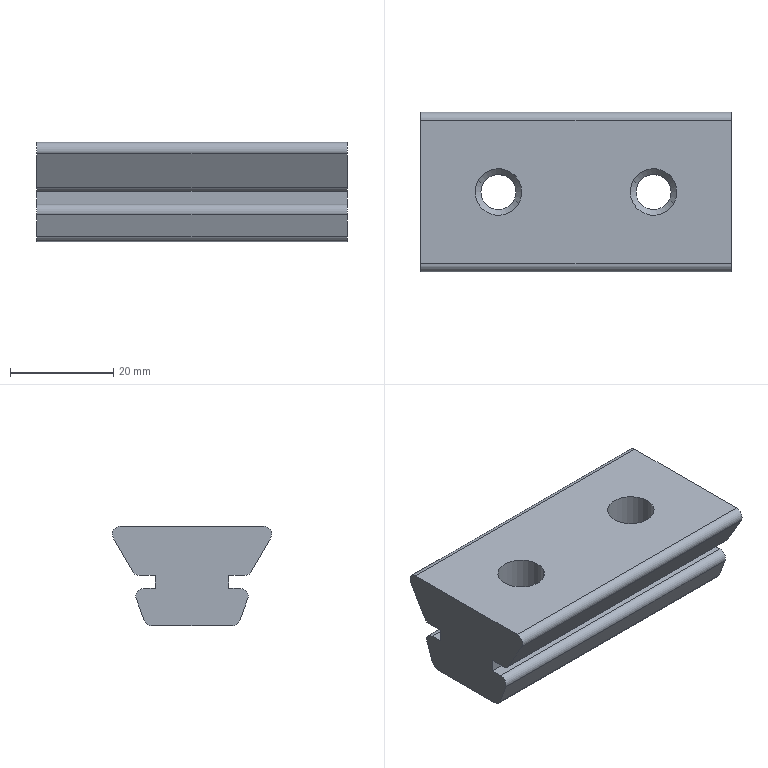Part | STEP file | 31E-01014QY25 | 1 solid | 34 faces | box 60 x 30.804 x 19.2 mm | volume 24408 mm3 | cylinder 16 | plane 14 | cone 4 | commonest cylinder face diameters 3 x8 6.8 x4 9 x4
STEP:
#1=CARTESIAN_POINT('',(0.,-7.1,-9.5));
#2=VERTEX_POINT('',#1);
#3=CARTESIAN_POINT('',(60.,-7.1,-9.5));
#4=VERTEX_POINT('',#3);
#5=CARTESIAN_POINT('',(30.,-7.1,-9.5));
#6=DIRECTION('',(1.,0.,0.));
#7=VECTOR('',#6,1.);
#8=LINE('',#5,#7);
#9=EDGE_CURVE('',#2,#4,#8,.T.);
#10=ORIENTED_EDGE('',*,*,#9,.F.);
#11=CARTESIAN_POINT('',(0.,-7.1,-12.));
#12=VERTEX_POINT('',#11);
#13=CARTESIAN_POINT('',(0.,-7.1,-10.75));
#14=DIRECTION('',(0.,0.,-1.));
#15=VECTOR('',#14,1.);
#16=LINE('',#13,#15);
#17=EDGE_CURVE('',#2,#12,#16,.T.);
#18=ORIENTED_EDGE('',*,*,#17,.T.);
#19=CARTESIAN_POINT('',(60.,-7.1,-12.));
#20=VERTEX_POINT('',#19);
#21=CARTESIAN_POINT('',(30.,-7.1,-12.));
#22=DIRECTION('',(1.,0.,0.));
#23=VECTOR('',#22,1.);
#24=LINE('',#21,#23);
#25=EDGE_CURVE('',#12,#20,#24,.T.);
#26=ORIENTED_EDGE('',*,*,#25,.T.);
#27=CARTESIAN_POINT('',(60.,-7.1,-10.75));
#28=DIRECTION('',(0.,0.,-1.));
#29=VECTOR('',#28,1.);
#30=LINE('',#27,#29);
#31=EDGE_CURVE('',#4,#20,#30,.T.);
#32=ORIENTED_EDGE('',*,*,#31,.F.);
#33=EDGE_LOOP('',(#10,#18,#26,#32));
#34=FACE_OUTER_BOUND('',#33,.T.);
#35=CARTESIAN_POINT('',(0.,-7.1,-9.5));
#36=DIRECTION('',(0.,-1.,0.));
#37=DIRECTION('',(0.,0.,-1.));
#38=AXIS2_PLACEMENT_3D('',#35,#36,#37);
#39=PLANE('',#38);
#40=ADVANCED_FACE('',(#34),#39,.T.);
#41=CARTESIAN_POINT('',(0.,7.1,-12.));
#42=VERTEX_POINT('',#41);
#43=CARTESIAN_POINT('',(60.,7.1,-12.));
#44=VERTEX_POINT('',#43);
#45=CARTESIAN_POINT('',(30.,7.1,-12.));
#46=DIRECTION('',(1.,0.,0.));
#47=VECTOR('',#46,1.);
#48=LINE('',#45,#47);
#49=EDGE_CURVE('',#42,#44,#48,.T.);
#50=ORIENTED_EDGE('',*,*,#49,.F.);
#51=CARTESIAN_POINT('',(0.,7.1,-9.5));
#52=VERTEX_POINT('',#51);
#53=CARTESIAN_POINT('',(0.,7.1,-10.75));
#54=DIRECTION('',(0.,0.,-1.));
#55=VECTOR('',#54,1.);
#56=LINE('',#53,#55);
#57=EDGE_CURVE('',#42,#52,#56,.F.);
#58=ORIENTED_EDGE('',*,*,#57,.T.);
#59=CARTESIAN_POINT('',(60.,7.1,-9.5));
#60=VERTEX_POINT('',#59);
#61=CARTESIAN_POINT('',(30.,7.1,-9.5));
#62=DIRECTION('',(1.,0.,0.));
#63=VECTOR('',#62,1.);
#64=LINE('',#61,#63);
#65=EDGE_CURVE('',#52,#60,#64,.T.);
#66=ORIENTED_EDGE('',*,*,#65,.T.);
#67=CARTESIAN_POINT('',(60.,7.1,-10.75));
#68=DIRECTION('',(0.,0.,-1.));
#69=VECTOR('',#68,1.);
#70=LINE('',#67,#69);
#71=EDGE_CURVE('',#44,#60,#70,.F.);
#72=ORIENTED_EDGE('',*,*,#71,.F.);
#73=EDGE_LOOP('',(#50,#58,#66,#72));
#74=FACE_OUTER_BOUND('',#73,.T.);
#75=CARTESIAN_POINT('',(0.,7.1,-9.5));
#76=DIRECTION('',(0.,-1.,0.));
#77=DIRECTION('',(0.,0.,-1.));
#78=AXIS2_PLACEMENT_3D('',#75,#76,#77);
#79=PLANE('',#78);
#80=ADVANCED_FACE('',(#74),#79,.F.);
#81=CARTESIAN_POINT('',(60.,13.902,0.));
#82=VERTEX_POINT('',#81);
#83=CARTESIAN_POINT('',(60.,15.201,-2.25));
#84=VERTEX_POINT('',#83);
#85=CARTESIAN_POINT('',(60.,13.902,-1.5));
#86=DIRECTION('',(1.,0.,0.));
#87=AXIS2_PLACEMENT_3D('',#85,#86,$);
#88=CIRCLE('',#87,1.5);
#89=EDGE_CURVE('',#82,#84,#88,.F.);
#90=ORIENTED_EDGE('',*,*,#89,.T.);
#91=CARTESIAN_POINT('',(0.,15.201,-2.25));
#92=VERTEX_POINT('',#91);
#93=CARTESIAN_POINT('',(30.,15.201,-2.25));
#94=DIRECTION('',(1.,0.,0.));
#95=VECTOR('',#94,1.);
#96=LINE('',#93,#95);
#97=EDGE_CURVE('',#92,#84,#96,.T.);
#98=ORIENTED_EDGE('',*,*,#97,.F.);
#99=CARTESIAN_POINT('',(0.,13.902,0.));
#100=VERTEX_POINT('',#99);
#101=CARTESIAN_POINT('',(0.,13.902,-1.5));
#102=DIRECTION('',(1.,0.,0.));
#103=AXIS2_PLACEMENT_3D('',#101,#102,$);
#104=CIRCLE('',#103,1.5);
#105=EDGE_CURVE('',#92,#100,#104,.T.);
#106=ORIENTED_EDGE('',*,*,#105,.T.);
#107=CARTESIAN_POINT('',(30.,13.902,0.));
#108=DIRECTION('',(1.,0.,0.));
#109=VECTOR('',#108,1.);
#110=LINE('',#107,#109);
#111=EDGE_CURVE('',#100,#82,#110,.T.);
#112=ORIENTED_EDGE('',*,*,#111,.T.);
#113=EDGE_LOOP('',(#90,#98,#106,#112));
#114=FACE_OUTER_BOUND('',#113,.T.);
#115=CARTESIAN_POINT('',(30.,13.902,-1.5));
#116=DIRECTION('',(1.,0.,0.));
#117=DIRECTION('',(0.,0.866,-0.5));
#118=AXIS2_PLACEMENT_3D('',#115,#116,#117);
#119=CYLINDRICAL_SURFACE('',#118,1.5);
#120=ADVANCED_FACE('',(#114),#119,.T.);
#121=CARTESIAN_POINT('',(60.,-15.201,-2.25));
#122=VERTEX_POINT('',#121);
#123=CARTESIAN_POINT('',(60.,-13.902,0.));
#124=VERTEX_POINT('',#123);
#125=CARTESIAN_POINT('',(60.,-13.902,-1.5));
#126=DIRECTION('',(1.,0.,0.));
#127=AXIS2_PLACEMENT_3D('',#125,#126,$);
#128=CIRCLE('',#127,1.5);
#129=EDGE_CURVE('',#122,#124,#128,.F.);
#130=ORIENTED_EDGE('',*,*,#129,.T.);
#131=CARTESIAN_POINT('',(0.,-13.902,0.));
#132=VERTEX_POINT('',#131);
#133=CARTESIAN_POINT('',(30.,-13.902,0.));
#134=DIRECTION('',(1.,0.,0.));
#135=VECTOR('',#134,1.);
#136=LINE('',#133,#135);
#137=EDGE_CURVE('',#132,#124,#136,.T.);
#138=ORIENTED_EDGE('',*,*,#137,.F.);
#139=CARTESIAN_POINT('',(0.,-15.201,-2.25));
#140=VERTEX_POINT('',#139);
#141=CARTESIAN_POINT('',(0.,-13.902,-1.5));
#142=DIRECTION('',(1.,0.,0.));
#143=AXIS2_PLACEMENT_3D('',#141,#142,$);
#144=CIRCLE('',#143,1.5);
#145=EDGE_CURVE('',#132,#140,#144,.T.);
#146=ORIENTED_EDGE('',*,*,#145,.T.);
#147=CARTESIAN_POINT('',(30.,-15.201,-2.25));
#148=DIRECTION('',(1.,0.,0.));
#149=VECTOR('',#148,1.);
#150=LINE('',#147,#149);
#151=EDGE_CURVE('',#140,#122,#150,.T.);
#152=ORIENTED_EDGE('',*,*,#151,.T.);
#153=EDGE_LOOP('',(#130,#138,#146,#152));
#154=FACE_OUTER_BOUND('',#153,.T.);
#155=CARTESIAN_POINT('',(30.,-13.902,-1.5));
#156=DIRECTION('',(1.,0.,0.));
#157=DIRECTION('',(0.,0.,1.));
#158=AXIS2_PLACEMENT_3D('',#155,#156,#157);
#159=CYLINDRICAL_SURFACE('',#158,1.5);
#160=ADVANCED_FACE('',(#154),#159,.T.);
#161=CARTESIAN_POINT('',(60.,10.149,-9.5));
#162=VERTEX_POINT('',#161);
#163=CARTESIAN_POINT('',(60.,8.625,-9.5));
#164=DIRECTION('',(0.,-1.,0.));
#165=VECTOR('',#164,1.);
#166=LINE('',#163,#165);
#167=EDGE_CURVE('',#60,#162,#166,.F.);
#168=ORIENTED_EDGE('',*,*,#167,.F.);
#169=ORIENTED_EDGE('',*,*,#65,.F.);
#170=CARTESIAN_POINT('',(0.,10.149,-9.5));
#171=VERTEX_POINT('',#170);
#172=CARTESIAN_POINT('',(0.,8.625,-9.5));
#173=DIRECTION('',(0.,-1.,0.));
#174=VECTOR('',#173,1.);
#175=LINE('',#172,#174);
#176=EDGE_CURVE('',#52,#171,#175,.F.);
#177=ORIENTED_EDGE('',*,*,#176,.T.);
#178=CARTESIAN_POINT('',(30.,10.149,-9.5));
#179=DIRECTION('',(1.,0.,0.));
#180=VECTOR('',#179,1.);
#181=LINE('',#178,#180);
#182=EDGE_CURVE('',#171,#162,#181,.T.);
#183=ORIENTED_EDGE('',*,*,#182,.T.);
#184=EDGE_LOOP('',(#168,#169,#177,#183));
#185=FACE_OUTER_BOUND('',#184,.T.);
#186=CARTESIAN_POINT('',(0.,-11.015,-9.5));
#187=DIRECTION('',(0.,0.,-1.));
#188=DIRECTION('',(0.,1.,0.));
#189=AXIS2_PLACEMENT_3D('',#186,#187,#188);
#190=PLANE('',#189);
#191=ADVANCED_FACE('',(#185),#190,.T.);
#192=CARTESIAN_POINT('',(0.,11.448,-8.75));
#193=VERTEX_POINT('',#192);
#194=CARTESIAN_POINT('',(60.,11.448,-8.75));
#195=VERTEX_POINT('',#194);
#196=CARTESIAN_POINT('',(30.,11.448,-8.75));
#197=DIRECTION('',(1.,0.,0.));
#198=VECTOR('',#197,1.);
#199=LINE('',#196,#198);
#200=EDGE_CURVE('',#193,#195,#199,.T.);
#201=ORIENTED_EDGE('',*,*,#200,.F.);
#202=CARTESIAN_POINT('',(0.,13.325,-5.5));
#203=DIRECTION('',(0.,-0.5,-0.866));
#204=VECTOR('',#203,1.);
#205=LINE('',#202,#204);
#206=EDGE_CURVE('',#193,#92,#205,.F.);
#207=ORIENTED_EDGE('',*,*,#206,.T.);
#208=ORIENTED_EDGE('',*,*,#97,.T.);
#209=CARTESIAN_POINT('',(60.,13.325,-5.5));
#210=DIRECTION('',(0.,-0.5,-0.866));
#211=VECTOR('',#210,1.);
#212=LINE('',#209,#211);
#213=EDGE_CURVE('',#195,#84,#212,.F.);
#214=ORIENTED_EDGE('',*,*,#213,.F.);
#215=EDGE_LOOP('',(#201,#207,#208,#214));
#216=FACE_OUTER_BOUND('',#215,.T.);
#217=CARTESIAN_POINT('',(0.,16.5,0.));
#218=DIRECTION('',(0.,-0.866,0.5));
#219=DIRECTION('',(0.,-0.5,-0.866));
#220=AXIS2_PLACEMENT_3D('',#217,#218,#219);
#221=PLANE('',#220);
#222=ADVANCED_FACE('',(#216),#221,.F.);
#223=CARTESIAN_POINT('',(60.,10.149,-8.));
#224=DIRECTION('',(1.,0.,0.));
#225=AXIS2_PLACEMENT_3D('',#223,#224,$);
#226=CIRCLE('',#225,1.5);
#227=EDGE_CURVE('',#195,#162,#226,.F.);
#228=ORIENTED_EDGE('',*,*,#227,.T.);
#229=ORIENTED_EDGE('',*,*,#182,.F.);
#230=CARTESIAN_POINT('',(0.,10.149,-8.));
#231=DIRECTION('',(1.,0.,0.));
#232=AXIS2_PLACEMENT_3D('',#230,#231,$);
#233=CIRCLE('',#232,1.5);
#234=EDGE_CURVE('',#171,#193,#233,.T.);
#235=ORIENTED_EDGE('',*,*,#234,.T.);
#236=ORIENTED_EDGE('',*,*,#200,.T.);
#237=EDGE_LOOP('',(#228,#229,#235,#236));
#238=FACE_OUTER_BOUND('',#237,.T.);
#239=CARTESIAN_POINT('',(30.,10.149,-8.));
#240=DIRECTION('',(1.,0.,0.));
#241=DIRECTION('',(0.,0.,-1.));
#242=AXIS2_PLACEMENT_3D('',#239,#240,#241);
#243=CYLINDRICAL_SURFACE('',#242,1.5);
#244=ADVANCED_FACE('',(#238),#243,.T.);
#245=CARTESIAN_POINT('',(0.,9.358,-12.));
#246=VERTEX_POINT('',#245);
#247=CARTESIAN_POINT('',(0.,8.229,-12.));
#248=DIRECTION('',(0.,1.,0.));
#249=VECTOR('',#248,1.);
#250=LINE('',#247,#249);
#251=EDGE_CURVE('',#246,#42,#250,.F.);
#252=ORIENTED_EDGE('',*,*,#251,.T.);
#253=ORIENTED_EDGE('',*,*,#49,.T.);
#254=CARTESIAN_POINT('',(60.,9.358,-12.));
#255=VERTEX_POINT('',#254);
#256=CARTESIAN_POINT('',(60.,8.229,-12.));
#257=DIRECTION('',(0.,1.,0.));
#258=VECTOR('',#257,1.);
#259=LINE('',#256,#258);
#260=EDGE_CURVE('',#255,#44,#259,.F.);
#261=ORIENTED_EDGE('',*,*,#260,.F.);
#262=CARTESIAN_POINT('',(30.,9.358,-12.));
#263=DIRECTION('',(1.,0.,0.));
#264=VECTOR('',#263,1.);
#265=LINE('',#262,#264);
#266=EDGE_CURVE('',#246,#255,#265,.T.);
#267=ORIENTED_EDGE('',*,*,#266,.F.);
#268=EDGE_LOOP('',(#252,#253,#261,#267));
#269=FACE_OUTER_BOUND('',#268,.T.);
#270=CARTESIAN_POINT('',(0.,-7.1,-12.));
#271=DIRECTION('',(0.,0.,1.));
#272=DIRECTION('',(0.,-1.,0.));
#273=AXIS2_PLACEMENT_3D('',#270,#271,#272);
#274=PLANE('',#273);
#275=ADVANCED_FACE('',(#269),#274,.T.);
#276=CARTESIAN_POINT('',(60.,10.767,-14.013));
#277=VERTEX_POINT('',#276);
#278=CARTESIAN_POINT('',(60.,9.358,-13.5));
#279=DIRECTION('',(1.,0.,0.));
#280=AXIS2_PLACEMENT_3D('',#278,#279,$);
#281=CIRCLE('',#280,1.5);
#282=EDGE_CURVE('',#255,#277,#281,.F.);
#283=ORIENTED_EDGE('',*,*,#282,.T.);
#284=CARTESIAN_POINT('',(0.,10.767,-14.013));
#285=VERTEX_POINT('',#284);
#286=CARTESIAN_POINT('',(30.,10.767,-14.013));
#287=DIRECTION('',(1.,0.,0.));
#288=VECTOR('',#287,1.);
#289=LINE('',#286,#288);
#290=EDGE_CURVE('',#285,#277,#289,.T.);
#291=ORIENTED_EDGE('',*,*,#290,.F.);
#292=CARTESIAN_POINT('',(0.,9.358,-13.5));
#293=DIRECTION('',(1.,0.,0.));
#294=AXIS2_PLACEMENT_3D('',#292,#293,$);
#295=CIRCLE('',#294,1.5);
#296=EDGE_CURVE('',#285,#246,#295,.T.);
#297=ORIENTED_EDGE('',*,*,#296,.T.);
#298=ORIENTED_EDGE('',*,*,#266,.T.);
#299=EDGE_LOOP('',(#283,#291,#297,#298));
#300=FACE_OUTER_BOUND('',#299,.T.);
#301=CARTESIAN_POINT('',(30.,9.358,-13.5));
#302=DIRECTION('',(1.,0.,0.));
#303=DIRECTION('',(0.,0.9397,-0.342));
#304=AXIS2_PLACEMENT_3D('',#301,#302,#303);
#305=CYLINDRICAL_SURFACE('',#304,1.5);
#306=ADVANCED_FACE('',(#300),#305,.T.);
#307=CARTESIAN_POINT('',(0.,9.239,-18.213));
#308=VERTEX_POINT('',#307);
#309=CARTESIAN_POINT('',(60.,9.239,-18.213));
#310=VERTEX_POINT('',#309);
#311=CARTESIAN_POINT('',(30.,9.239,-18.213));
#312=DIRECTION('',(1.,0.,0.));
#313=VECTOR('',#312,1.);
#314=LINE('',#311,#313);
#315=EDGE_CURVE('',#308,#310,#314,.T.);
#316=ORIENTED_EDGE('',*,*,#315,.F.);
#317=CARTESIAN_POINT('',(0.,10.003,-16.113));
#318=DIRECTION('',(0.,-0.342,-0.9397));
#319=VECTOR('',#318,1.);
#320=LINE('',#317,#319);
#321=EDGE_CURVE('',#308,#285,#320,.F.);
#322=ORIENTED_EDGE('',*,*,#321,.T.);
#323=ORIENTED_EDGE('',*,*,#290,.T.);
#324=CARTESIAN_POINT('',(60.,10.003,-16.113));
#325=DIRECTION('',(0.,-0.342,-0.9397));
#326=VECTOR('',#325,1.);
#327=LINE('',#324,#326);
#328=EDGE_CURVE('',#310,#277,#327,.F.);
#329=ORIENTED_EDGE('',*,*,#328,.F.);
#330=EDGE_LOOP('',(#316,#322,#323,#329));
#331=FACE_OUTER_BOUND('',#330,.T.);
#332=CARTESIAN_POINT('',(0.,11.5,-12.));
#333=DIRECTION('',(0.,-0.9397,0.342));
#334=DIRECTION('',(0.,-0.342,-0.9397));
#335=AXIS2_PLACEMENT_3D('',#332,#333,#334);
#336=PLANE('',#335);
#337=ADVANCED_FACE('',(#331),#336,.F.);
#338=CARTESIAN_POINT('',(60.,7.829,-19.2));
#339=VERTEX_POINT('',#338);
#340=CARTESIAN_POINT('',(60.,7.829,-17.7));
#341=DIRECTION('',(1.,0.,0.));
#342=AXIS2_PLACEMENT_3D('',#340,#341,$);
#343=CIRCLE('',#342,1.5);
#344=EDGE_CURVE('',#310,#339,#343,.F.);
#345=ORIENTED_EDGE('',*,*,#344,.T.);
#346=CARTESIAN_POINT('',(0.,7.829,-19.2));
#347=VERTEX_POINT('',#346);
#348=CARTESIAN_POINT('',(30.,7.829,-19.2));
#349=DIRECTION('',(1.,0.,0.));
#350=VECTOR('',#349,1.);
#351=LINE('',#348,#350);
#352=EDGE_CURVE('',#347,#339,#351,.T.);
#353=ORIENTED_EDGE('',*,*,#352,.F.);
#354=CARTESIAN_POINT('',(0.,7.829,-17.7));
#355=DIRECTION('',(1.,0.,0.));
#356=AXIS2_PLACEMENT_3D('',#354,#355,$);
#357=CIRCLE('',#356,1.5);
#358=EDGE_CURVE('',#347,#308,#357,.T.);
#359=ORIENTED_EDGE('',*,*,#358,.T.);
#360=ORIENTED_EDGE('',*,*,#315,.T.);
#361=EDGE_LOOP('',(#345,#353,#359,#360));
#362=FACE_OUTER_BOUND('',#361,.T.);
#363=CARTESIAN_POINT('',(30.,7.829,-17.7));
#364=DIRECTION('',(1.,0.,0.));
#365=DIRECTION('',(0.,0.,-1.));
#366=AXIS2_PLACEMENT_3D('',#363,#364,#365);
#367=CYLINDRICAL_SURFACE('',#366,1.5);
#368=ADVANCED_FACE('',(#362),#367,.T.);
#369=CARTESIAN_POINT('',(60.,-7.829,-19.2));
#370=VERTEX_POINT('',#369);
#371=CARTESIAN_POINT('',(60.,-9.239,-18.213));
#372=VERTEX_POINT('',#371);
#373=CARTESIAN_POINT('',(60.,-7.829,-17.7));
#374=DIRECTION('',(1.,0.,0.));
#375=AXIS2_PLACEMENT_3D('',#373,#374,$);
#376=CIRCLE('',#375,1.5);
#377=EDGE_CURVE('',#370,#372,#376,.F.);
#378=ORIENTED_EDGE('',*,*,#377,.T.);
#379=CARTESIAN_POINT('',(0.,-9.239,-18.213));
#380=VERTEX_POINT('',#379);
#381=CARTESIAN_POINT('',(30.,-9.239,-18.213));
#382=DIRECTION('',(1.,0.,0.));
#383=VECTOR('',#382,1.);
#384=LINE('',#381,#383);
#385=EDGE_CURVE('',#380,#372,#384,.T.);
#386=ORIENTED_EDGE('',*,*,#385,.F.);
#387=CARTESIAN_POINT('',(0.,-7.829,-19.2));
#388=VERTEX_POINT('',#387);
#389=CARTESIAN_POINT('',(0.,-7.829,-17.7));
#390=DIRECTION('',(1.,0.,0.));
#391=AXIS2_PLACEMENT_3D('',#389,#390,$);
#392=CIRCLE('',#391,1.5);
#393=EDGE_CURVE('',#380,#388,#392,.T.);
#394=ORIENTED_EDGE('',*,*,#393,.T.);
#395=CARTESIAN_POINT('',(30.,-7.829,-19.2));
#396=DIRECTION('',(1.,0.,0.));
#397=VECTOR('',#396,1.);
#398=LINE('',#395,#397);
#399=EDGE_CURVE('',#388,#370,#398,.T.);
#400=ORIENTED_EDGE('',*,*,#399,.T.);
#401=EDGE_LOOP('',(#378,#386,#394,#400));
#402=FACE_OUTER_BOUND('',#401,.T.);
#403=CARTESIAN_POINT('',(30.,-7.829,-17.7));
#404=DIRECTION('',(1.,0.,0.));
#405=DIRECTION('',(0.,-0.9397,-0.342));
#406=AXIS2_PLACEMENT_3D('',#403,#404,#405);
#407=CYLINDRICAL_SURFACE('',#406,1.5);
#408=ADVANCED_FACE('',(#402),#407,.T.);
#409=CARTESIAN_POINT('',(60.,-9.358,-12.));
#410=VERTEX_POINT('',#409);
#411=CARTESIAN_POINT('',(60.,-8.229,-12.));
#412=DIRECTION('',(0.,-1.,0.));
#413=VECTOR('',#412,1.);
#414=LINE('',#411,#413);
#415=EDGE_CURVE('',#20,#410,#414,.T.);
#416=ORIENTED_EDGE('',*,*,#415,.F.);
#417=ORIENTED_EDGE('',*,*,#25,.F.);
#418=CARTESIAN_POINT('',(0.,-9.358,-12.));
#419=VERTEX_POINT('',#418);
#420=CARTESIAN_POINT('',(0.,-8.229,-12.));
#421=DIRECTION('',(0.,-1.,0.));
#422=VECTOR('',#421,1.);
#423=LINE('',#420,#422);
#424=EDGE_CURVE('',#12,#419,#423,.T.);
#425=ORIENTED_EDGE('',*,*,#424,.T.);
#426=CARTESIAN_POINT('',(30.,-9.358,-12.));
#427=DIRECTION('',(1.,0.,0.));
#428=VECTOR('',#427,1.);
#429=LINE('',#426,#428);
#430=EDGE_CURVE('',#419,#410,#429,.T.);
#431=ORIENTED_EDGE('',*,*,#430,.T.);
#432=EDGE_LOOP('',(#416,#417,#425,#431));
#433=FACE_OUTER_BOUND('',#432,.T.);
#434=ADVANCED_FACE('',(#433),#274,.T.);
#435=CARTESIAN_POINT('',(0.,-10.767,-14.013));
#436=VERTEX_POINT('',#435);
#437=CARTESIAN_POINT('',(0.,-10.003,-16.113));
#438=DIRECTION('',(0.,0.342,-0.9397));
#439=VECTOR('',#438,1.);
#440=LINE('',#437,#439);
#441=EDGE_CURVE('',#436,#380,#440,.T.);
#442=ORIENTED_EDGE('',*,*,#441,.T.);
#443=ORIENTED_EDGE('',*,*,#385,.T.);
#444=CARTESIAN_POINT('',(60.,-10.767,-14.013));
#445=VERTEX_POINT('',#444);
#446=CARTESIAN_POINT('',(60.,-10.003,-16.113));
#447=DIRECTION('',(0.,0.342,-0.9397));
#448=VECTOR('',#447,1.);
#449=LINE('',#446,#448);
#450=EDGE_CURVE('',#445,#372,#449,.T.);
#451=ORIENTED_EDGE('',*,*,#450,.F.);
#452=CARTESIAN_POINT('',(30.,-10.767,-14.013));
#453=DIRECTION('',(1.,0.,0.));
#454=VECTOR('',#453,1.);
#455=LINE('',#452,#454);
#456=EDGE_CURVE('',#436,#445,#455,.T.);
#457=ORIENTED_EDGE('',*,*,#456,.F.);
#458=EDGE_LOOP('',(#442,#443,#451,#457));
#459=FACE_OUTER_BOUND('',#458,.T.);
#460=CARTESIAN_POINT('',(0.,-11.5,-12.));
#461=DIRECTION('',(0.,-0.9397,-0.342));
#462=DIRECTION('',(0.,0.342,-0.9397));
#463=AXIS2_PLACEMENT_3D('',#460,#461,#462);
#464=PLANE('',#463);
#465=ADVANCED_FACE('',(#459),#464,.T.);
#466=CARTESIAN_POINT('',(60.,-9.358,-13.5));
#467=DIRECTION('',(1.,0.,0.));
#468=AXIS2_PLACEMENT_3D('',#466,#467,$);
#469=CIRCLE('',#468,1.5);
#470=EDGE_CURVE('',#445,#410,#469,.F.);
#471=ORIENTED_EDGE('',*,*,#470,.T.);
#472=ORIENTED_EDGE('',*,*,#430,.F.);
#473=CARTESIAN_POINT('',(0.,-9.358,-13.5));
#474=DIRECTION('',(1.,0.,0.));
#475=AXIS2_PLACEMENT_3D('',#473,#474,$);
#476=CIRCLE('',#475,1.5);
#477=EDGE_CURVE('',#419,#436,#476,.T.);
#478=ORIENTED_EDGE('',*,*,#477,.T.);
#479=ORIENTED_EDGE('',*,*,#456,.T.);
#480=EDGE_LOOP('',(#471,#472,#478,#479));
#481=FACE_OUTER_BOUND('',#480,.T.);
#482=CARTESIAN_POINT('',(30.,-9.358,-13.5));
#483=DIRECTION('',(1.,0.,0.));
#484=DIRECTION('',(0.,0.,1.));
#485=AXIS2_PLACEMENT_3D('',#482,#483,#484);
#486=CYLINDRICAL_SURFACE('',#485,1.5);
#487=ADVANCED_FACE('',(#481),#486,.T.);
#488=CARTESIAN_POINT('',(0.,-10.149,-9.5));
#489=VERTEX_POINT('',#488);
#490=CARTESIAN_POINT('',(0.,-8.625,-9.5));
#491=DIRECTION('',(0.,1.,0.));
#492=VECTOR('',#491,1.);
#493=LINE('',#490,#492);
#494=EDGE_CURVE('',#489,#2,#493,.T.);
#495=ORIENTED_EDGE('',*,*,#494,.T.);
#496=ORIENTED_EDGE('',*,*,#9,.T.);
#497=CARTESIAN_POINT('',(60.,-10.149,-9.5));
#498=VERTEX_POINT('',#497);
#499=CARTESIAN_POINT('',(60.,-8.625,-9.5));
#500=DIRECTION('',(0.,1.,0.));
#501=VECTOR('',#500,1.);
#502=LINE('',#499,#501);
#503=EDGE_CURVE('',#498,#4,#502,.T.);
#504=ORIENTED_EDGE('',*,*,#503,.F.);
#505=CARTESIAN_POINT('',(30.,-10.149,-9.5));
#506=DIRECTION('',(1.,0.,0.));
#507=VECTOR('',#506,1.);
#508=LINE('',#505,#507);
#509=EDGE_CURVE('',#489,#498,#508,.T.);
#510=ORIENTED_EDGE('',*,*,#509,.F.);
#511=EDGE_LOOP('',(#495,#496,#504,#510));
#512=FACE_OUTER_BOUND('',#511,.T.);
#513=ADVANCED_FACE('',(#512),#190,.T.);
#514=CARTESIAN_POINT('',(60.,-11.448,-8.75));
#515=VERTEX_POINT('',#514);
#516=CARTESIAN_POINT('',(60.,-13.325,-5.5));
#517=DIRECTION('',(0.,0.5,-0.866));
#518=VECTOR('',#517,1.);
#519=LINE('',#516,#518);
#520=EDGE_CURVE('',#122,#515,#519,.T.);
#521=ORIENTED_EDGE('',*,*,#520,.F.);
#522=ORIENTED_EDGE('',*,*,#151,.F.);
#523=CARTESIAN_POINT('',(0.,-11.448,-8.75));
#524=VERTEX_POINT('',#523);
#525=CARTESIAN_POINT('',(0.,-13.325,-5.5));
#526=DIRECTION('',(0.,0.5,-0.866));
#527=VECTOR('',#526,1.);
#528=LINE('',#525,#527);
#529=EDGE_CURVE('',#140,#524,#528,.T.);
#530=ORIENTED_EDGE('',*,*,#529,.T.);
#531=CARTESIAN_POINT('',(30.,-11.448,-8.75));
#532=DIRECTION('',(1.,0.,0.));
#533=VECTOR('',#532,1.);
#534=LINE('',#531,#533);
#535=EDGE_CURVE('',#524,#515,#534,.T.);
#536=ORIENTED_EDGE('',*,*,#535,.T.);
#537=EDGE_LOOP('',(#521,#522,#530,#536));
#538=FACE_OUTER_BOUND('',#537,.T.);
#539=CARTESIAN_POINT('',(0.,-16.5,0.));
#540=DIRECTION('',(0.,-0.866,-0.5));
#541=DIRECTION('',(0.,0.5,-0.866));
#542=AXIS2_PLACEMENT_3D('',#539,#540,#541);
#543=PLANE('',#542);
#544=ADVANCED_FACE('',(#538),#543,.T.);
#545=CARTESIAN_POINT('',(0.,-10.149,-8.));
#546=DIRECTION('',(1.,0.,0.));
#547=AXIS2_PLACEMENT_3D('',#545,#546,$);
#548=CIRCLE('',#547,1.5);
#549=EDGE_CURVE('',#524,#489,#548,.T.);
#550=ORIENTED_EDGE('',*,*,#549,.F.);
#551=ORIENTED_EDGE('',*,*,#529,.F.);
#552=ORIENTED_EDGE('',*,*,#145,.F.);
#553=CARTESIAN_POINT('',(0.,0.,0.));
#554=DIRECTION('',(0.,1.,0.));
#555=VECTOR('',#554,1.);
#556=LINE('',#553,#555);
#557=EDGE_CURVE('',#100,#132,#556,.F.);
#558=ORIENTED_EDGE('',*,*,#557,.F.);
#559=ORIENTED_EDGE('',*,*,#105,.F.);
#560=ORIENTED_EDGE('',*,*,#206,.F.);
#561=ORIENTED_EDGE('',*,*,#234,.F.);
#562=ORIENTED_EDGE('',*,*,#176,.F.);
#563=ORIENTED_EDGE('',*,*,#57,.F.);
#564=ORIENTED_EDGE('',*,*,#251,.F.);
#565=ORIENTED_EDGE('',*,*,#296,.F.);
#566=ORIENTED_EDGE('',*,*,#321,.F.);
#567=ORIENTED_EDGE('',*,*,#358,.F.);
#568=CARTESIAN_POINT('',(0.,0.,-19.2));
#569=DIRECTION('',(0.,-1.,0.));
#570=VECTOR('',#569,1.);
#571=LINE('',#568,#570);
#572=EDGE_CURVE('',#388,#347,#571,.F.);
#573=ORIENTED_EDGE('',*,*,#572,.F.);
#574=ORIENTED_EDGE('',*,*,#393,.F.);
#575=ORIENTED_EDGE('',*,*,#441,.F.);
#576=ORIENTED_EDGE('',*,*,#477,.F.);
#577=ORIENTED_EDGE('',*,*,#424,.F.);
#578=ORIENTED_EDGE('',*,*,#17,.F.);
#579=ORIENTED_EDGE('',*,*,#494,.F.);
#580=EDGE_LOOP('',(#550,#551,#552,#558,#559,#560,#561,#562,#563,#564,#565,#566,#567,#573,#574,#575,#576,#577,#578,#579));
#581=FACE_OUTER_BOUND('',#580,.T.);
#582=CARTESIAN_POINT('',(0.,0.,0.));
#583=DIRECTION('',(1.,0.,0.));
#584=DIRECTION('',(0.,1.,0.));
#585=AXIS2_PLACEMENT_3D('',#582,#583,#584);
#586=PLANE('',#585);
#587=ADVANCED_FACE('',(#581),#586,.F.);
#588=ORIENTED_EDGE('',*,*,#503,.T.);
#589=ORIENTED_EDGE('',*,*,#31,.T.);
#590=ORIENTED_EDGE('',*,*,#415,.T.);
#591=ORIENTED_EDGE('',*,*,#470,.F.);
#592=ORIENTED_EDGE('',*,*,#450,.T.);
#593=ORIENTED_EDGE('',*,*,#377,.F.);
#594=CARTESIAN_POINT('',(60.,0.,-19.2));
#595=DIRECTION('',(0.,-1.,0.));
#596=VECTOR('',#595,1.);
#597=LINE('',#594,#596);
#598=EDGE_CURVE('',#370,#339,#597,.F.);
#599=ORIENTED_EDGE('',*,*,#598,.T.);
#600=ORIENTED_EDGE('',*,*,#344,.F.);
#601=ORIENTED_EDGE('',*,*,#328,.T.);
#602=ORIENTED_EDGE('',*,*,#282,.F.);
#603=ORIENTED_EDGE('',*,*,#260,.T.);
#604=ORIENTED_EDGE('',*,*,#71,.T.);
#605=ORIENTED_EDGE('',*,*,#167,.T.);
#606=ORIENTED_EDGE('',*,*,#227,.F.);
#607=ORIENTED_EDGE('',*,*,#213,.T.);
#608=ORIENTED_EDGE('',*,*,#89,.F.);
#609=CARTESIAN_POINT('',(60.,0.,0.));
#610=DIRECTION('',(0.,1.,0.));
#611=VECTOR('',#610,1.);
#612=LINE('',#609,#611);
#613=EDGE_CURVE('',#82,#124,#612,.F.);
#614=ORIENTED_EDGE('',*,*,#613,.T.);
#615=ORIENTED_EDGE('',*,*,#129,.F.);
#616=ORIENTED_EDGE('',*,*,#520,.T.);
#617=CARTESIAN_POINT('',(60.,-10.149,-8.));
#618=DIRECTION('',(1.,0.,0.));
#619=AXIS2_PLACEMENT_3D('',#617,#618,$);
#620=CIRCLE('',#619,1.5);
#621=EDGE_CURVE('',#498,#515,#620,.F.);
#622=ORIENTED_EDGE('',*,*,#621,.F.);
#623=EDGE_LOOP('',(#588,#589,#590,#591,#592,#593,#599,#600,#601,#602,#603,#604,#605,#606,#607,#608,#614,#615,#616,#622));
#624=FACE_OUTER_BOUND('',#623,.T.);
#625=CARTESIAN_POINT('',(60.,0.,0.));
#626=DIRECTION('',(1.,0.,0.));
#627=DIRECTION('',(0.,1.,0.));
#628=AXIS2_PLACEMENT_3D('',#625,#626,#627);
#629=PLANE('',#628);
#630=ADVANCED_FACE('',(#624),#629,.T.);
#631=ORIENTED_EDGE('',*,*,#621,.T.);
#632=ORIENTED_EDGE('',*,*,#535,.F.);
#633=ORIENTED_EDGE('',*,*,#549,.T.);
#634=ORIENTED_EDGE('',*,*,#509,.T.);
#635=EDGE_LOOP('',(#631,#632,#633,#634));
#636=FACE_OUTER_BOUND('',#635,.T.);
#637=CARTESIAN_POINT('',(30.,-10.149,-8.));
#638=DIRECTION('',(1.,0.,0.));
#639=DIRECTION('',(0.,-0.866,-0.5));
#640=AXIS2_PLACEMENT_3D('',#637,#638,#639);
#641=CYLINDRICAL_SURFACE('',#640,1.5);
#642=ADVANCED_FACE('',(#636),#641,.T.);
#643=ORIENTED_EDGE('',*,*,#399,.F.);
#644=ORIENTED_EDGE('',*,*,#572,.T.);
#645=ORIENTED_EDGE('',*,*,#352,.T.);
#646=ORIENTED_EDGE('',*,*,#598,.F.);
#647=EDGE_LOOP('',(#643,#644,#645,#646));
#648=FACE_OUTER_BOUND('',#647,.T.);
#649=CARTESIAN_POINT('',(17.984,-1.63,-19.2));
#650=VERTEX_POINT('',#649);
#651=CARTESIAN_POINT('',(12.016,1.63,-19.2));
#652=VERTEX_POINT('',#651);
#653=CARTESIAN_POINT('',(15.,0.,-19.2));
#654=DIRECTION('',(0.,0.,1.));
#655=AXIS2_PLACEMENT_3D('',#653,#654,$);
#656=CIRCLE('',#655,3.4);
#657=EDGE_CURVE('',#650,#652,#656,.T.);
#658=ORIENTED_EDGE('',*,*,#657,.T.);
#659=CARTESIAN_POINT('',(15.,0.,-19.2));
#660=DIRECTION('',(0.,0.,1.));
#661=AXIS2_PLACEMENT_3D('',#659,#660,$);
#662=CIRCLE('',#661,3.4);
#663=EDGE_CURVE('',#652,#650,#662,.T.);
#664=ORIENTED_EDGE('',*,*,#663,.T.);
#665=EDGE_LOOP('',(#658,#664));
#666=FACE_BOUND('',#665,.T.);
#667=CARTESIAN_POINT('',(47.984,-1.63,-19.2));
#668=VERTEX_POINT('',#667);
#669=CARTESIAN_POINT('',(42.016,1.63,-19.2));
#670=VERTEX_POINT('',#669);
#671=CARTESIAN_POINT('',(45.,0.,-19.2));
#672=DIRECTION('',(0.,0.,1.));
#673=AXIS2_PLACEMENT_3D('',#671,#672,$);
#674=CIRCLE('',#673,3.4);
#675=EDGE_CURVE('',#668,#670,#674,.T.);
#676=ORIENTED_EDGE('',*,*,#675,.T.);
#677=CARTESIAN_POINT('',(45.,0.,-19.2));
#678=DIRECTION('',(0.,0.,1.));
#679=AXIS2_PLACEMENT_3D('',#677,#678,$);
#680=CIRCLE('',#679,3.4);
#681=EDGE_CURVE('',#670,#668,#680,.T.);
#682=ORIENTED_EDGE('',*,*,#681,.T.);
#683=EDGE_LOOP('',(#676,#682));
#684=FACE_BOUND('',#683,.T.);
#685=CARTESIAN_POINT('',(0.,8.879,-19.2));
#686=DIRECTION('',(0.,0.,1.));
#687=DIRECTION('',(0.,-1.,0.));
#688=AXIS2_PLACEMENT_3D('',#685,#686,#687);
#689=PLANE('',#688);
#690=ADVANCED_FACE('',(#648,#666,#684),#689,.F.);
#691=ORIENTED_EDGE('',*,*,#137,.T.);
#692=ORIENTED_EDGE('',*,*,#613,.F.);
#693=ORIENTED_EDGE('',*,*,#111,.F.);
#694=ORIENTED_EDGE('',*,*,#557,.T.);
#695=EDGE_LOOP('',(#691,#692,#693,#694));
#696=FACE_OUTER_BOUND('',#695,.T.);
#697=CARTESIAN_POINT('',(18.949,-2.157,0.));
#698=VERTEX_POINT('',#697);
#699=CARTESIAN_POINT('',(11.051,2.157,0.));
#700=VERTEX_POINT('',#699);
#701=CARTESIAN_POINT('',(15.,0.,0.));
#702=DIRECTION('',(0.,0.,-1.));
#703=AXIS2_PLACEMENT_3D('',#701,#702,$);
#704=CIRCLE('',#703,4.5);
#705=EDGE_CURVE('',#698,#700,#704,.T.);
#706=ORIENTED_EDGE('',*,*,#705,.T.);
#707=CARTESIAN_POINT('',(15.,0.,0.));
#708=DIRECTION('',(0.,0.,-1.));
#709=AXIS2_PLACEMENT_3D('',#707,#708,$);
#710=CIRCLE('',#709,4.5);
#711=EDGE_CURVE('',#700,#698,#710,.T.);
#712=ORIENTED_EDGE('',*,*,#711,.T.);
#713=EDGE_LOOP('',(#706,#712));
#714=FACE_BOUND('',#713,.T.);
#715=CARTESIAN_POINT('',(48.949,-2.157,0.));
#716=VERTEX_POINT('',#715);
#717=CARTESIAN_POINT('',(41.051,2.157,0.));
#718=VERTEX_POINT('',#717);
#719=CARTESIAN_POINT('',(45.,0.,0.));
#720=DIRECTION('',(0.,0.,-1.));
#721=AXIS2_PLACEMENT_3D('',#719,#720,$);
#722=CIRCLE('',#721,4.5);
#723=EDGE_CURVE('',#716,#718,#722,.T.);
#724=ORIENTED_EDGE('',*,*,#723,.T.);
#725=CARTESIAN_POINT('',(45.,0.,0.));
#726=DIRECTION('',(0.,0.,-1.));
#727=AXIS2_PLACEMENT_3D('',#725,#726,$);
#728=CIRCLE('',#727,4.5);
#729=EDGE_CURVE('',#718,#716,#728,.T.);
#730=ORIENTED_EDGE('',*,*,#729,.T.);
#731=EDGE_LOOP('',(#724,#730));
#732=FACE_BOUND('',#731,.T.);
#733=CARTESIAN_POINT('',(0.,-16.5,0.));
#734=DIRECTION('',(0.,0.,-1.));
#735=DIRECTION('',(0.,1.,0.));
#736=AXIS2_PLACEMENT_3D('',#733,#734,#735);
#737=PLANE('',#736);
#738=ADVANCED_FACE('',(#696,#714,#732),#737,.F.);
#739=CARTESIAN_POINT('',(42.016,1.63,-9.1));
#740=VERTEX_POINT('',#739);
#741=CARTESIAN_POINT('',(41.051,2.157,-8.));
#742=VERTEX_POINT('',#741);
#743=CARTESIAN_POINT('',(41.534,1.894,-8.55));
#744=DIRECTION('',(-0.6205,0.339,0.7071));
#745=VECTOR('',#744,1.);
#746=LINE('',#743,#745);
#747=EDGE_CURVE('',#740,#742,#746,.T.);
#748=ORIENTED_EDGE('',*,*,#747,.T.);
#749=CARTESIAN_POINT('',(48.949,-2.157,-8.));
#750=VERTEX_POINT('',#749);
#751=CARTESIAN_POINT('',(45.,0.,-8.));
#752=DIRECTION('',(0.,0.,1.));
#753=AXIS2_PLACEMENT_3D('',#751,#752,$);
#754=CIRCLE('',#753,4.5);
#755=EDGE_CURVE('',#750,#742,#754,.F.);
#756=ORIENTED_EDGE('',*,*,#755,.F.);
#757=CARTESIAN_POINT('',(47.984,-1.63,-9.1));
#758=VERTEX_POINT('',#757);
#759=CARTESIAN_POINT('',(48.466,-1.894,-8.55));
#760=DIRECTION('',(0.6205,-0.339,0.7071));
#761=VECTOR('',#760,1.);
#762=LINE('',#759,#761);
#763=EDGE_CURVE('',#758,#750,#762,.T.);
#764=ORIENTED_EDGE('',*,*,#763,.F.);
#765=CARTESIAN_POINT('',(45.,0.,-9.1));
#766=DIRECTION('',(0.,0.,1.));
#767=AXIS2_PLACEMENT_3D('',#765,#766,$);
#768=CIRCLE('',#767,3.4);
#769=EDGE_CURVE('',#758,#740,#768,.F.);
#770=ORIENTED_EDGE('',*,*,#769,.T.);
#771=EDGE_LOOP('',(#748,#756,#764,#770));
#772=FACE_OUTER_BOUND('',#771,.T.);
#773=CARTESIAN_POINT('',(45.,0.,-9.1));
#774=DIRECTION('',(0.,0.,1.));
#775=DIRECTION('',(0.8776,-0.4794,0.));
#776=AXIS2_PLACEMENT_3D('',#773,#774,#775);
#777=CONICAL_SURFACE('',#776,3.4,0.7854);
#778=ADVANCED_FACE('',(#772),#777,.F.);
#779=ORIENTED_EDGE('',*,*,#681,.F.);
#780=CARTESIAN_POINT('',(42.016,1.63,-14.55));
#781=DIRECTION('',(0.,0.,-1.));
#782=VECTOR('',#781,1.);
#783=LINE('',#780,#782);
#784=EDGE_CURVE('',#670,#740,#783,.F.);
#785=ORIENTED_EDGE('',*,*,#784,.T.);
#786=ORIENTED_EDGE('',*,*,#769,.F.);
#787=CARTESIAN_POINT('',(47.984,-1.63,-14.55));
#788=DIRECTION('',(0.,0.,-1.));
#789=VECTOR('',#788,1.);
#790=LINE('',#787,#789);
#791=EDGE_CURVE('',#668,#758,#790,.F.);
#792=ORIENTED_EDGE('',*,*,#791,.F.);
#793=EDGE_LOOP('',(#779,#785,#786,#792));
#794=FACE_OUTER_BOUND('',#793,.T.);
#795=CARTESIAN_POINT('',(45.,0.,-0.1));
#796=DIRECTION('',(0.,0.,-1.));
#797=DIRECTION('',(0.8776,-0.4794,0.));
#798=AXIS2_PLACEMENT_3D('',#795,#796,#797);
#799=CYLINDRICAL_SURFACE('',#798,3.4);
#800=ADVANCED_FACE('',(#794),#799,.F.);
#801=ORIENTED_EDGE('',*,*,#763,.T.);
#802=CARTESIAN_POINT('',(45.,0.,-8.));
#803=DIRECTION('',(0.,0.,1.));
#804=AXIS2_PLACEMENT_3D('',#802,#803,$);
#805=CIRCLE('',#804,4.5);
#806=EDGE_CURVE('',#742,#750,#805,.F.);
#807=ORIENTED_EDGE('',*,*,#806,.F.);
#808=ORIENTED_EDGE('',*,*,#747,.F.);
#809=CARTESIAN_POINT('',(45.,0.,-9.1));
#810=DIRECTION('',(0.,0.,1.));
#811=AXIS2_PLACEMENT_3D('',#809,#810,$);
#812=CIRCLE('',#811,3.4);
#813=EDGE_CURVE('',#740,#758,#812,.F.);
#814=ORIENTED_EDGE('',*,*,#813,.T.);
#815=EDGE_LOOP('',(#801,#807,#808,#814));
#816=FACE_OUTER_BOUND('',#815,.T.);
#817=ADVANCED_FACE('',(#816),#777,.F.);
#818=ORIENTED_EDGE('',*,*,#723,.F.);
#819=CARTESIAN_POINT('',(48.949,-2.157,-3.8));
#820=DIRECTION('',(0.,0.,-1.));
#821=VECTOR('',#820,1.);
#822=LINE('',#819,#821);
#823=EDGE_CURVE('',#750,#716,#822,.F.);
#824=ORIENTED_EDGE('',*,*,#823,.F.);
#825=ORIENTED_EDGE('',*,*,#755,.T.);
#826=CARTESIAN_POINT('',(41.051,2.157,-3.8));
#827=DIRECTION('',(0.,0.,-1.));
#828=VECTOR('',#827,1.);
#829=LINE('',#826,#828);
#830=EDGE_CURVE('',#742,#718,#829,.F.);
#831=ORIENTED_EDGE('',*,*,#830,.T.);
#832=EDGE_LOOP('',(#818,#824,#825,#831));
#833=FACE_OUTER_BOUND('',#832,.T.);
#834=CARTESIAN_POINT('',(45.,0.,-0.1));
#835=DIRECTION('',(0.,0.,-1.));
#836=DIRECTION('',(0.8776,-0.4794,0.));
#837=AXIS2_PLACEMENT_3D('',#834,#835,#836);
#838=CYLINDRICAL_SURFACE('',#837,4.5);
#839=ADVANCED_FACE('',(#833),#838,.F.);
#840=ORIENTED_EDGE('',*,*,#675,.F.);
#841=ORIENTED_EDGE('',*,*,#791,.T.);
#842=ORIENTED_EDGE('',*,*,#813,.F.);
#843=ORIENTED_EDGE('',*,*,#784,.F.);
#844=EDGE_LOOP('',(#840,#841,#842,#843));
#845=FACE_OUTER_BOUND('',#844,.T.);
#846=ADVANCED_FACE('',(#845),#799,.F.);
#847=ORIENTED_EDGE('',*,*,#729,.F.);
#848=ORIENTED_EDGE('',*,*,#830,.F.);
#849=ORIENTED_EDGE('',*,*,#806,.T.);
#850=ORIENTED_EDGE('',*,*,#823,.T.);
#851=EDGE_LOOP('',(#847,#848,#849,#850));
#852=FACE_OUTER_BOUND('',#851,.T.);
#853=ADVANCED_FACE('',(#852),#838,.F.);
#854=CARTESIAN_POINT('',(12.016,1.63,-9.1));
#855=VERTEX_POINT('',#854);
#856=CARTESIAN_POINT('',(11.051,2.157,-8.));
#857=VERTEX_POINT('',#856);
#858=CARTESIAN_POINT('',(11.534,1.894,-8.55));
#859=DIRECTION('',(-0.6205,0.339,0.7071));
#860=VECTOR('',#859,1.);
#861=LINE('',#858,#860);
#862=EDGE_CURVE('',#855,#857,#861,.T.);
#863=ORIENTED_EDGE('',*,*,#862,.T.);
#864=CARTESIAN_POINT('',(18.949,-2.157,-8.));
#865=VERTEX_POINT('',#864);
#866=CARTESIAN_POINT('',(15.,0.,-8.));
#867=DIRECTION('',(0.,0.,1.));
#868=AXIS2_PLACEMENT_3D('',#866,#867,$);
#869=CIRCLE('',#868,4.5);
#870=EDGE_CURVE('',#865,#857,#869,.F.);
#871=ORIENTED_EDGE('',*,*,#870,.F.);
#872=CARTESIAN_POINT('',(17.984,-1.63,-9.1));
#873=VERTEX_POINT('',#872);
#874=CARTESIAN_POINT('',(18.466,-1.894,-8.55));
#875=DIRECTION('',(0.6205,-0.339,0.7071));
#876=VECTOR('',#875,1.);
#877=LINE('',#874,#876);
#878=EDGE_CURVE('',#873,#865,#877,.T.);
#879=ORIENTED_EDGE('',*,*,#878,.F.);
#880=CARTESIAN_POINT('',(15.,0.,-9.1));
#881=DIRECTION('',(0.,0.,1.));
#882=AXIS2_PLACEMENT_3D('',#880,#881,$);
#883=CIRCLE('',#882,3.4);
#884=EDGE_CURVE('',#873,#855,#883,.F.);
#885=ORIENTED_EDGE('',*,*,#884,.T.);
#886=EDGE_LOOP('',(#863,#871,#879,#885));
#887=FACE_OUTER_BOUND('',#886,.T.);
#888=CARTESIAN_POINT('',(15.,0.,-9.1));
#889=DIRECTION('',(0.,0.,1.));
#890=DIRECTION('',(0.8776,-0.4794,0.));
#891=AXIS2_PLACEMENT_3D('',#888,#889,#890);
#892=CONICAL_SURFACE('',#891,3.4,0.7854);
#893=ADVANCED_FACE('',(#887),#892,.F.);
#894=ORIENTED_EDGE('',*,*,#663,.F.);
#895=CARTESIAN_POINT('',(12.016,1.63,-14.55));
#896=DIRECTION('',(0.,0.,-1.));
#897=VECTOR('',#896,1.);
#898=LINE('',#895,#897);
#899=EDGE_CURVE('',#652,#855,#898,.F.);
#900=ORIENTED_EDGE('',*,*,#899,.T.);
#901=ORIENTED_EDGE('',*,*,#884,.F.);
#902=CARTESIAN_POINT('',(17.984,-1.63,-14.55));
#903=DIRECTION('',(0.,0.,-1.));
#904=VECTOR('',#903,1.);
#905=LINE('',#902,#904);
#906=EDGE_CURVE('',#650,#873,#905,.F.);
#907=ORIENTED_EDGE('',*,*,#906,.F.);
#908=EDGE_LOOP('',(#894,#900,#901,#907));
#909=FACE_OUTER_BOUND('',#908,.T.);
#910=CARTESIAN_POINT('',(15.,0.,-0.1));
#911=DIRECTION('',(0.,0.,-1.));
#912=DIRECTION('',(0.8776,-0.4794,0.));
#913=AXIS2_PLACEMENT_3D('',#910,#911,#912);
#914=CYLINDRICAL_SURFACE('',#913,3.4);
#915=ADVANCED_FACE('',(#909),#914,.F.);
#916=ORIENTED_EDGE('',*,*,#878,.T.);
#917=CARTESIAN_POINT('',(15.,0.,-8.));
#918=DIRECTION('',(0.,0.,1.));
#919=AXIS2_PLACEMENT_3D('',#917,#918,$);
#920=CIRCLE('',#919,4.5);
#921=EDGE_CURVE('',#857,#865,#920,.F.);
#922=ORIENTED_EDGE('',*,*,#921,.F.);
#923=ORIENTED_EDGE('',*,*,#862,.F.);
#924=CARTESIAN_POINT('',(15.,0.,-9.1));
#925=DIRECTION('',(0.,0.,1.));
#926=AXIS2_PLACEMENT_3D('',#924,#925,$);
#927=CIRCLE('',#926,3.4);
#928=EDGE_CURVE('',#855,#873,#927,.F.);
#929=ORIENTED_EDGE('',*,*,#928,.T.);
#930=EDGE_LOOP('',(#916,#922,#923,#929));
#931=FACE_OUTER_BOUND('',#930,.T.);
#932=ADVANCED_FACE('',(#931),#892,.F.);
#933=ORIENTED_EDGE('',*,*,#705,.F.);
#934=CARTESIAN_POINT('',(18.949,-2.157,-3.8));
#935=DIRECTION('',(0.,0.,-1.));
#936=VECTOR('',#935,1.);
#937=LINE('',#934,#936);
#938=EDGE_CURVE('',#865,#698,#937,.F.);
#939=ORIENTED_EDGE('',*,*,#938,.F.);
#940=ORIENTED_EDGE('',*,*,#870,.T.);
#941=CARTESIAN_POINT('',(11.051,2.157,-3.8));
#942=DIRECTION('',(0.,0.,-1.));
#943=VECTOR('',#942,1.);
#944=LINE('',#941,#943);
#945=EDGE_CURVE('',#857,#700,#944,.F.);
#946=ORIENTED_EDGE('',*,*,#945,.T.);
#947=EDGE_LOOP('',(#933,#939,#940,#946));
#948=FACE_OUTER_BOUND('',#947,.T.);
#949=CARTESIAN_POINT('',(15.,0.,-0.1));
#950=DIRECTION('',(0.,0.,-1.));
#951=DIRECTION('',(0.8776,-0.4794,0.));
#952=AXIS2_PLACEMENT_3D('',#949,#950,#951);
#953=CYLINDRICAL_SURFACE('',#952,4.5);
#954=ADVANCED_FACE('',(#948),#953,.F.);
#955=ORIENTED_EDGE('',*,*,#657,.F.);
#956=ORIENTED_EDGE('',*,*,#906,.T.);
#957=ORIENTED_EDGE('',*,*,#928,.F.);
#958=ORIENTED_EDGE('',*,*,#899,.F.);
#959=EDGE_LOOP('',(#955,#956,#957,#958));
#960=FACE_OUTER_BOUND('',#959,.T.);
#961=ADVANCED_FACE('',(#960),#914,.F.);
#962=ORIENTED_EDGE('',*,*,#711,.F.);
#963=ORIENTED_EDGE('',*,*,#945,.F.);
#964=ORIENTED_EDGE('',*,*,#921,.T.);
#965=ORIENTED_EDGE('',*,*,#938,.T.);
#966=EDGE_LOOP('',(#962,#963,#964,#965));
#967=FACE_OUTER_BOUND('',#966,.T.);
#968=ADVANCED_FACE('',(#967),#953,.F.);
#969=CLOSED_SHELL('',(#40,#80,#120,#160,#191,#222,#244,#275,#306,#337,#368,#408,#434,#465,#487,#513,#544,#587,#630,#642,#690,#738,#778,#800,#817,#839,#846,#853,#893,#915,#932,#954,#961,#968));
#970=MANIFOLD_SOLID_BREP('',#969);
#971=(LENGTH_UNIT()NAMED_UNIT(*)SI_UNIT(.MILLI.,.METRE.));
#972=UNCERTAINTY_MEASURE_WITH_UNIT(LENGTH_MEASURE(0.005),#971,'','');
#973=(NAMED_UNIT(*)PLANE_ANGLE_UNIT()SI_UNIT($,.RADIAN.));
#974=(NAMED_UNIT(*)SI_UNIT($,.STERADIAN.)SOLID_ANGLE_UNIT());
#975=(GEOMETRIC_REPRESENTATION_CONTEXT(3)GLOBAL_UNCERTAINTY_ASSIGNED_CONTEXT((#972))GLOBAL_UNIT_ASSIGNED_CONTEXT((#971,#973,#974))REPRESENTATION_CONTEXT('',''));
#976=ADVANCED_BREP_SHAPE_REPRESENTATION('',(#970),#975);